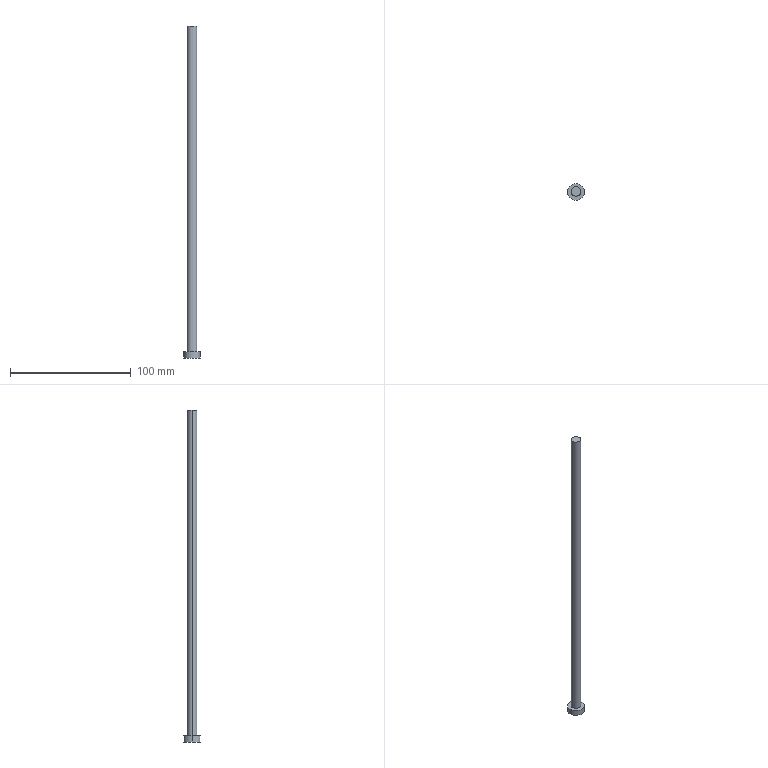Part | Creo | 1 solid | 7 faces | box 14 x 14 x 274.665 mm | volume 14325 mm3 | cylinder 4 | plane 3 | commonest cylinder face diameters 8 x2 14 x2
STEP:
#1=CARTESIAN_POINT('',(-74.,235.,39.165));
#2=VERTEX_POINT('',#1);
#3=CARTESIAN_POINT('',(-66.,235.,39.165));
#4=VERTEX_POINT('',#3);
#5=CARTESIAN_POINT('',(-70.,235.,39.165));
#6=DIRECTION('',(0.,0.,1.));
#7=DIRECTION('',(-1.,0.,0.));
#8=AXIS2_PLACEMENT_3D('',#5,#6,#7);
#9=CIRCLE('',#8,4.);
#10=EDGE_CURVE('',#2,#4,#9,.T.);
#11=ORIENTED_EDGE('',*,*,#10,.T.);
#12=CARTESIAN_POINT('',(-66.,235.,-230.5));
#13=VERTEX_POINT('',#12);
#14=CARTESIAN_POINT('',(-66.,235.,39.165));
#15=DIRECTION('',(0.,0.,-1.));
#16=VECTOR('',#15,269.665);
#17=LINE('',#14,#16);
#18=EDGE_CURVE('',#4,#13,#17,.T.);
#19=ORIENTED_EDGE('',*,*,#18,.T.);
#20=CARTESIAN_POINT('',(-74.,235.,-230.5));
#21=VERTEX_POINT('',#20);
#22=CARTESIAN_POINT('',(-70.,235.,-230.5));
#23=DIRECTION('',(0.,0.,-1.));
#24=DIRECTION('',(1.,0.,0.));
#25=AXIS2_PLACEMENT_3D('',#22,#23,#24);
#26=CIRCLE('',#25,4.);
#27=EDGE_CURVE('',#13,#21,#26,.T.);
#28=ORIENTED_EDGE('',*,*,#27,.T.);
#29=CARTESIAN_POINT('',(-74.,235.,39.165));
#30=DIRECTION('',(0.,0.,-1.));
#31=VECTOR('',#30,269.665);
#32=LINE('',#29,#31);
#33=EDGE_CURVE('',#2,#21,#32,.T.);
#34=ORIENTED_EDGE('',*,*,#33,.F.);
#35=EDGE_LOOP('',(#11,#19,#28,#34));
#36=FACE_OUTER_BOUND('',#35,.F.);
#37=CARTESIAN_POINT('',(-70.,235.,49.5));
#38=DIRECTION('',(0.,0.,-1.));
#39=DIRECTION('',(1.,0.,0.));
#40=AXIS2_PLACEMENT_3D('',#37,#38,#39);
#41=CYLINDRICAL_SURFACE('',#40,4.);
#42=ADVANCED_FACE('',(#36),#41,.T.);
#43=ORIENTED_EDGE('',*,*,#10,.F.);
#44=CARTESIAN_POINT('',(-70.,235.,39.165));
#45=DIRECTION('',(0.,0.,1.));
#46=DIRECTION('',(1.,0.,0.));
#47=AXIS2_PLACEMENT_3D('',#44,#45,#46);
#48=CIRCLE('',#47,4.);
#49=EDGE_CURVE('',#4,#2,#48,.T.);
#50=ORIENTED_EDGE('',*,*,#49,.F.);
#51=EDGE_LOOP('',(#43,#50));
#52=FACE_OUTER_BOUND('',#51,.F.);
#53=CARTESIAN_POINT('',(0.,0.,39.165));
#54=DIRECTION('',(0.,0.,-1.));
#55=DIRECTION('',(0.,1.,0.));
#56=AXIS2_PLACEMENT_3D('',#53,#54,#55);
#57=PLANE('',#56);
#58=ADVANCED_FACE('',(#52),#57,.F.);
#59=ORIENTED_EDGE('',*,*,#49,.T.);
#60=ORIENTED_EDGE('',*,*,#33,.T.);
#61=CARTESIAN_POINT('',(-70.,235.,-230.5));
#62=DIRECTION('',(0.,0.,-1.));
#63=DIRECTION('',(-1.,0.,0.));
#64=AXIS2_PLACEMENT_3D('',#61,#62,#63);
#65=CIRCLE('',#64,4.);
#66=EDGE_CURVE('',#21,#13,#65,.T.);
#67=ORIENTED_EDGE('',*,*,#66,.T.);
#68=ORIENTED_EDGE('',*,*,#18,.F.);
#69=EDGE_LOOP('',(#59,#60,#67,#68));
#70=FACE_OUTER_BOUND('',#69,.F.);
#71=CARTESIAN_POINT('',(-70.,235.,49.5));
#72=DIRECTION('',(0.,0.,-1.));
#73=DIRECTION('',(1.,0.,0.));
#74=AXIS2_PLACEMENT_3D('',#71,#72,#73);
#75=CYLINDRICAL_SURFACE('',#74,4.);
#76=ADVANCED_FACE('',(#70),#75,.T.);
#77=CARTESIAN_POINT('',(-63.,235.,-230.5));
#78=VERTEX_POINT('',#77);
#79=CARTESIAN_POINT('',(-77.,235.,-230.5));
#80=VERTEX_POINT('',#79);
#81=CARTESIAN_POINT('',(-70.,235.,-230.5));
#82=DIRECTION('',(0.,0.,1.));
#83=DIRECTION('',(1.,0.,0.));
#84=AXIS2_PLACEMENT_3D('',#81,#82,#83);
#85=CIRCLE('',#84,7.);
#86=EDGE_CURVE('',#78,#80,#85,.T.);
#87=ORIENTED_EDGE('',*,*,#86,.F.);
#88=CARTESIAN_POINT('',(-70.,235.,-230.5));
#89=DIRECTION('',(0.,0.,1.));
#90=DIRECTION('',(-1.,0.,0.));
#91=AXIS2_PLACEMENT_3D('',#88,#89,#90);
#92=CIRCLE('',#91,7.);
#93=EDGE_CURVE('',#80,#78,#92,.T.);
#94=ORIENTED_EDGE('',*,*,#93,.F.);
#95=EDGE_LOOP('',(#87,#94));
#96=FACE_OUTER_BOUND('',#95,.F.);
#97=ORIENTED_EDGE('',*,*,#27,.F.);
#98=ORIENTED_EDGE('',*,*,#66,.F.);
#99=EDGE_LOOP('',(#97,#98));
#100=FACE_BOUND('',#99,.F.);
#101=CARTESIAN_POINT('',(-70.,235.,-230.5));
#102=DIRECTION('',(0.,0.,-1.));
#103=DIRECTION('',(1.,0.,0.));
#104=AXIS2_PLACEMENT_3D('',#101,#102,#103);
#105=PLANE('',#104);
#106=ADVANCED_FACE('',(#96,#100),#105,.F.);
#107=CARTESIAN_POINT('',(-77.,235.,-235.5));
#108=VERTEX_POINT('',#107);
#109=CARTESIAN_POINT('',(-63.,235.,-235.5));
#110=VERTEX_POINT('',#109);
#111=CARTESIAN_POINT('',(-70.,235.,-235.5));
#112=DIRECTION('',(0.,0.,-1.));
#113=DIRECTION('',(-1.,0.,0.));
#114=AXIS2_PLACEMENT_3D('',#111,#112,#113);
#115=CIRCLE('',#114,7.);
#116=EDGE_CURVE('',#108,#110,#115,.T.);
#117=ORIENTED_EDGE('',*,*,#116,.T.);
#118=CARTESIAN_POINT('',(-63.,235.,-230.5));
#119=DIRECTION('',(0.,0.,-1.));
#120=VECTOR('',#119,5.);
#121=LINE('',#118,#120);
#122=EDGE_CURVE('',#78,#110,#121,.T.);
#123=ORIENTED_EDGE('',*,*,#122,.F.);
#124=ORIENTED_EDGE('',*,*,#86,.T.);
#125=CARTESIAN_POINT('',(-77.,235.,-230.5));
#126=DIRECTION('',(0.,0.,-1.));
#127=VECTOR('',#126,5.);
#128=LINE('',#125,#127);
#129=EDGE_CURVE('',#80,#108,#128,.T.);
#130=ORIENTED_EDGE('',*,*,#129,.T.);
#131=EDGE_LOOP('',(#117,#123,#124,#130));
#132=FACE_OUTER_BOUND('',#131,.F.);
#133=CARTESIAN_POINT('',(-70.,235.,-245.913));
#134=DIRECTION('',(0.,0.,-1.));
#135=DIRECTION('',(1.,0.,0.));
#136=AXIS2_PLACEMENT_3D('',#133,#134,#135);
#137=CYLINDRICAL_SURFACE('',#136,7.);
#138=ADVANCED_FACE('',(#132),#137,.T.);
#139=CARTESIAN_POINT('',(-70.,235.,-235.5));
#140=DIRECTION('',(0.,0.,-1.));
#141=DIRECTION('',(1.,0.,0.));
#142=AXIS2_PLACEMENT_3D('',#139,#140,#141);
#143=CIRCLE('',#142,7.);
#144=EDGE_CURVE('',#110,#108,#143,.T.);
#145=ORIENTED_EDGE('',*,*,#144,.F.);
#146=ORIENTED_EDGE('',*,*,#116,.F.);
#147=EDGE_LOOP('',(#145,#146));
#148=FACE_OUTER_BOUND('',#147,.F.);
#149=CARTESIAN_POINT('',(-74.,235.,-235.5));
#150=DIRECTION('',(0.,0.,1.));
#151=DIRECTION('',(-1.,0.,0.));
#152=AXIS2_PLACEMENT_3D('',#149,#150,#151);
#153=PLANE('',#152);
#154=ADVANCED_FACE('',(#148),#153,.F.);
#155=ORIENTED_EDGE('',*,*,#144,.T.);
#156=ORIENTED_EDGE('',*,*,#129,.F.);
#157=ORIENTED_EDGE('',*,*,#93,.T.);
#158=ORIENTED_EDGE('',*,*,#122,.T.);
#159=EDGE_LOOP('',(#155,#156,#157,#158));
#160=FACE_OUTER_BOUND('',#159,.F.);
#161=CARTESIAN_POINT('',(-70.,235.,-245.913));
#162=DIRECTION('',(0.,0.,-1.));
#163=DIRECTION('',(1.,0.,0.));
#164=AXIS2_PLACEMENT_3D('',#161,#162,#163);
#165=CYLINDRICAL_SURFACE('',#164,7.);
#166=ADVANCED_FACE('',(#160),#165,.T.);
#167=CLOSED_SHELL('',(#42,#58,#76,#106,#138,#154,#166));
#168=MANIFOLD_SOLID_BREP('',#167);
#169=(LENGTH_UNIT()NAMED_UNIT(*)SI_UNIT(.MILLI.,.METRE.));
#170=UNCERTAINTY_MEASURE_WITH_UNIT(LENGTH_MEASURE(0.02754),#169,'','');
#171=(NAMED_UNIT(*)PLANE_ANGLE_UNIT()SI_UNIT($,.RADIAN.));
#172=PLANE_ANGLE_MEASURE_WITH_UNIT(PLANE_ANGLE_MEASURE(0.01745),#171);
#173=(CONVERSION_BASED_UNIT('DEGREE',#172)NAMED_UNIT(*)PLANE_ANGLE_UNIT());
#174=(NAMED_UNIT(*)SI_UNIT($,.STERADIAN.)SOLID_ANGLE_UNIT());
#175=(GEOMETRIC_REPRESENTATION_CONTEXT(3)GLOBAL_UNCERTAINTY_ASSIGNED_CONTEXT((#170))GLOBAL_UNIT_ASSIGNED_CONTEXT((#169,#173,#174))REPRESENTATION_CONTEXT('',''));
#176=ADVANCED_BREP_SHAPE_REPRESENTATION('',(#168),#175);